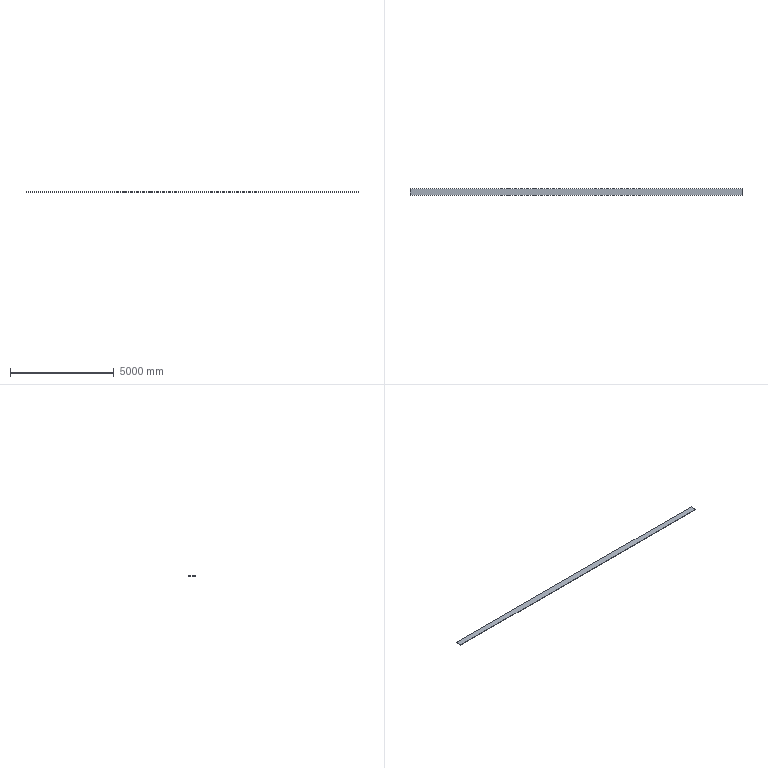Part | SolidWorks | features Extrusion 1 | 1 solid | 6 faces | box 16000 x 300 x 20 mm | volume 96000000 mm3 | plane 6
STEP:
#1=CARTESIAN_POINT('',(8000.,-150.,0.));
#2=VERTEX_POINT('',#1);
#3=CARTESIAN_POINT('',(8000.,150.,0.));
#4=VERTEX_POINT('',#3);
#5=CARTESIAN_POINT('',(8000.,150.,0.));
#6=DIRECTION('',(0.,1.,0.));
#7=VECTOR('',#6,1000.);
#8=LINE('',#5,#7);
#9=EDGE_CURVE('',#2,#4,#8,.T.);
#10=ORIENTED_EDGE('',*,*,#9,.T.);
#11=CARTESIAN_POINT('',(8000.,150.,20.));
#12=VERTEX_POINT('',#11);
#13=CARTESIAN_POINT('',(8000.,150.,20.));
#14=DIRECTION('',(0.,0.,-1.));
#15=VECTOR('',#14,1000.);
#16=LINE('',#13,#15);
#17=EDGE_CURVE('',#12,#4,#16,.T.);
#18=ORIENTED_EDGE('',*,*,#17,.F.);
#19=CARTESIAN_POINT('',(8000.,-150.,20.));
#20=VERTEX_POINT('',#19);
#21=CARTESIAN_POINT('',(8000.,150.,20.));
#22=DIRECTION('',(0.,1.,0.));
#23=VECTOR('',#22,1000.);
#24=LINE('',#21,#23);
#25=EDGE_CURVE('',#20,#12,#24,.T.);
#26=ORIENTED_EDGE('',*,*,#25,.F.);
#27=CARTESIAN_POINT('',(8000.,-150.,20.));
#28=DIRECTION('',(0.,0.,-1.));
#29=VECTOR('',#28,1000.);
#30=LINE('',#27,#29);
#31=EDGE_CURVE('',#20,#2,#30,.T.);
#32=ORIENTED_EDGE('',*,*,#31,.T.);
#33=EDGE_LOOP('',(#10,#18,#26,#32));
#34=FACE_OUTER_BOUND('',#33,.T.);
#35=CARTESIAN_POINT('',(8000.,150.,20.));
#36=DIRECTION('',(-1.,0.,0.));
#37=DIRECTION('',(0.,0.,1.));
#38=AXIS2_PLACEMENT_3D('',#35,#36,#37);
#39=PLANE('',#38);
#40=ADVANCED_FACE('',(#34),#39,.F.);
#41=CARTESIAN_POINT('',(-8000.,150.,0.));
#42=VERTEX_POINT('',#41);
#43=CARTESIAN_POINT('',(-8000.,150.,0.));
#44=DIRECTION('',(-1.,0.,0.));
#45=VECTOR('',#44,1000.);
#46=LINE('',#43,#45);
#47=EDGE_CURVE('',#4,#42,#46,.T.);
#48=ORIENTED_EDGE('',*,*,#47,.T.);
#49=CARTESIAN_POINT('',(-8000.,150.,20.));
#50=VERTEX_POINT('',#49);
#51=CARTESIAN_POINT('',(-8000.,150.,20.));
#52=DIRECTION('',(0.,0.,-1.));
#53=VECTOR('',#52,1000.);
#54=LINE('',#51,#53);
#55=EDGE_CURVE('',#50,#42,#54,.T.);
#56=ORIENTED_EDGE('',*,*,#55,.F.);
#57=CARTESIAN_POINT('',(-8000.,150.,20.));
#58=DIRECTION('',(-1.,0.,0.));
#59=VECTOR('',#58,1000.);
#60=LINE('',#57,#59);
#61=EDGE_CURVE('',#12,#50,#60,.T.);
#62=ORIENTED_EDGE('',*,*,#61,.F.);
#63=ORIENTED_EDGE('',*,*,#17,.T.);
#64=EDGE_LOOP('',(#48,#56,#62,#63));
#65=FACE_OUTER_BOUND('',#64,.T.);
#66=CARTESIAN_POINT('',(-8000.,150.,20.));
#67=DIRECTION('',(0.,-1.,0.));
#68=DIRECTION('',(0.,0.,-1.));
#69=AXIS2_PLACEMENT_3D('',#66,#67,#68);
#70=PLANE('',#69);
#71=ADVANCED_FACE('',(#65),#70,.F.);
#72=CARTESIAN_POINT('',(-8000.,-150.,0.));
#73=VERTEX_POINT('',#72);
#74=CARTESIAN_POINT('',(-8000.,150.,0.));
#75=DIRECTION('',(0.,-1.,0.));
#76=VECTOR('',#75,1000.);
#77=LINE('',#74,#76);
#78=EDGE_CURVE('',#42,#73,#77,.T.);
#79=ORIENTED_EDGE('',*,*,#78,.T.);
#80=CARTESIAN_POINT('',(-8000.,-150.,20.));
#81=VERTEX_POINT('',#80);
#82=CARTESIAN_POINT('',(-8000.,-150.,20.));
#83=DIRECTION('',(0.,0.,-1.));
#84=VECTOR('',#83,1000.);
#85=LINE('',#82,#84);
#86=EDGE_CURVE('',#81,#73,#85,.T.);
#87=ORIENTED_EDGE('',*,*,#86,.F.);
#88=CARTESIAN_POINT('',(-8000.,150.,20.));
#89=DIRECTION('',(0.,-1.,0.));
#90=VECTOR('',#89,1000.);
#91=LINE('',#88,#90);
#92=EDGE_CURVE('',#50,#81,#91,.T.);
#93=ORIENTED_EDGE('',*,*,#92,.F.);
#94=ORIENTED_EDGE('',*,*,#55,.T.);
#95=EDGE_LOOP('',(#79,#87,#93,#94));
#96=FACE_OUTER_BOUND('',#95,.T.);
#97=CARTESIAN_POINT('',(-8000.,150.,20.));
#98=DIRECTION('',(1.,0.,0.));
#99=DIRECTION('',(0.,0.,-1.));
#100=AXIS2_PLACEMENT_3D('',#97,#98,#99);
#101=PLANE('',#100);
#102=ADVANCED_FACE('',(#96),#101,.F.);
#103=CARTESIAN_POINT('',(-8000.,-150.,0.));
#104=DIRECTION('',(1.,0.,0.));
#105=VECTOR('',#104,1000.);
#106=LINE('',#103,#105);
#107=EDGE_CURVE('',#73,#2,#106,.T.);
#108=ORIENTED_EDGE('',*,*,#107,.T.);
#109=ORIENTED_EDGE('',*,*,#31,.F.);
#110=CARTESIAN_POINT('',(-8000.,-150.,20.));
#111=DIRECTION('',(1.,0.,0.));
#112=VECTOR('',#111,1000.);
#113=LINE('',#110,#112);
#114=EDGE_CURVE('',#81,#20,#113,.T.);
#115=ORIENTED_EDGE('',*,*,#114,.F.);
#116=ORIENTED_EDGE('',*,*,#86,.T.);
#117=EDGE_LOOP('',(#108,#109,#115,#116));
#118=FACE_OUTER_BOUND('',#117,.T.);
#119=CARTESIAN_POINT('',(-8000.,-150.,20.));
#120=DIRECTION('',(0.,1.,0.));
#121=DIRECTION('',(0.,0.,1.));
#122=AXIS2_PLACEMENT_3D('',#119,#120,#121);
#123=PLANE('',#122);
#124=ADVANCED_FACE('',(#118),#123,.F.);
#125=ORIENTED_EDGE('',*,*,#25,.T.);
#126=ORIENTED_EDGE('',*,*,#61,.T.);
#127=ORIENTED_EDGE('',*,*,#92,.T.);
#128=ORIENTED_EDGE('',*,*,#114,.T.);
#129=EDGE_LOOP('',(#125,#126,#127,#128));
#130=FACE_OUTER_BOUND('',#129,.T.);
#131=CARTESIAN_POINT('',(0.,0.,20.));
#132=DIRECTION('',(0.,0.,1.));
#133=DIRECTION('',(1.,0.,0.));
#134=AXIS2_PLACEMENT_3D('',#131,#132,#133);
#135=PLANE('',#134);
#136=ADVANCED_FACE('',(#130),#135,.T.);
#137=ORIENTED_EDGE('',*,*,#9,.F.);
#138=ORIENTED_EDGE('',*,*,#107,.F.);
#139=ORIENTED_EDGE('',*,*,#78,.F.);
#140=ORIENTED_EDGE('',*,*,#47,.F.);
#141=EDGE_LOOP('',(#137,#138,#139,#140));
#142=FACE_OUTER_BOUND('',#141,.T.);
#143=CARTESIAN_POINT('',(0.,0.,0.));
#144=DIRECTION('',(0.,0.,1.));
#145=DIRECTION('',(1.,0.,0.));
#146=AXIS2_PLACEMENT_3D('',#143,#144,#145);
#147=PLANE('',#146);
#148=ADVANCED_FACE('',(#142),#147,.F.);
#149=CLOSED_SHELL('',(#40,#71,#102,#124,#136,#148));
#150=MANIFOLD_SOLID_BREP('',#149);
#151=CARTESIAN_POINT('',(0.,0.,0.));
#152=DIRECTION('',(0.,0.,1.));
#153=DIRECTION('',(1.,0.,0.));
#154=AXIS2_PLACEMENT_3D('',#151,#152,#153);
#155=(LENGTH_UNIT()NAMED_UNIT(*)SI_UNIT(.MILLI.,.METRE.));
#156=UNCERTAINTY_MEASURE_WITH_UNIT(LENGTH_MEASURE(0.00001),#155,'','');
#157=(NAMED_UNIT(*)PLANE_ANGLE_UNIT()SI_UNIT($,.RADIAN.));
#158=(NAMED_UNIT(*)SI_UNIT($,.STERADIAN.)SOLID_ANGLE_UNIT());
#159=(GEOMETRIC_REPRESENTATION_CONTEXT(3)GLOBAL_UNCERTAINTY_ASSIGNED_CONTEXT((#156))GLOBAL_UNIT_ASSIGNED_CONTEXT((#155,#157,#158))REPRESENTATION_CONTEXT('',''));
#160=ADVANCED_BREP_SHAPE_REPRESENTATION('',(#150,#154),#159);